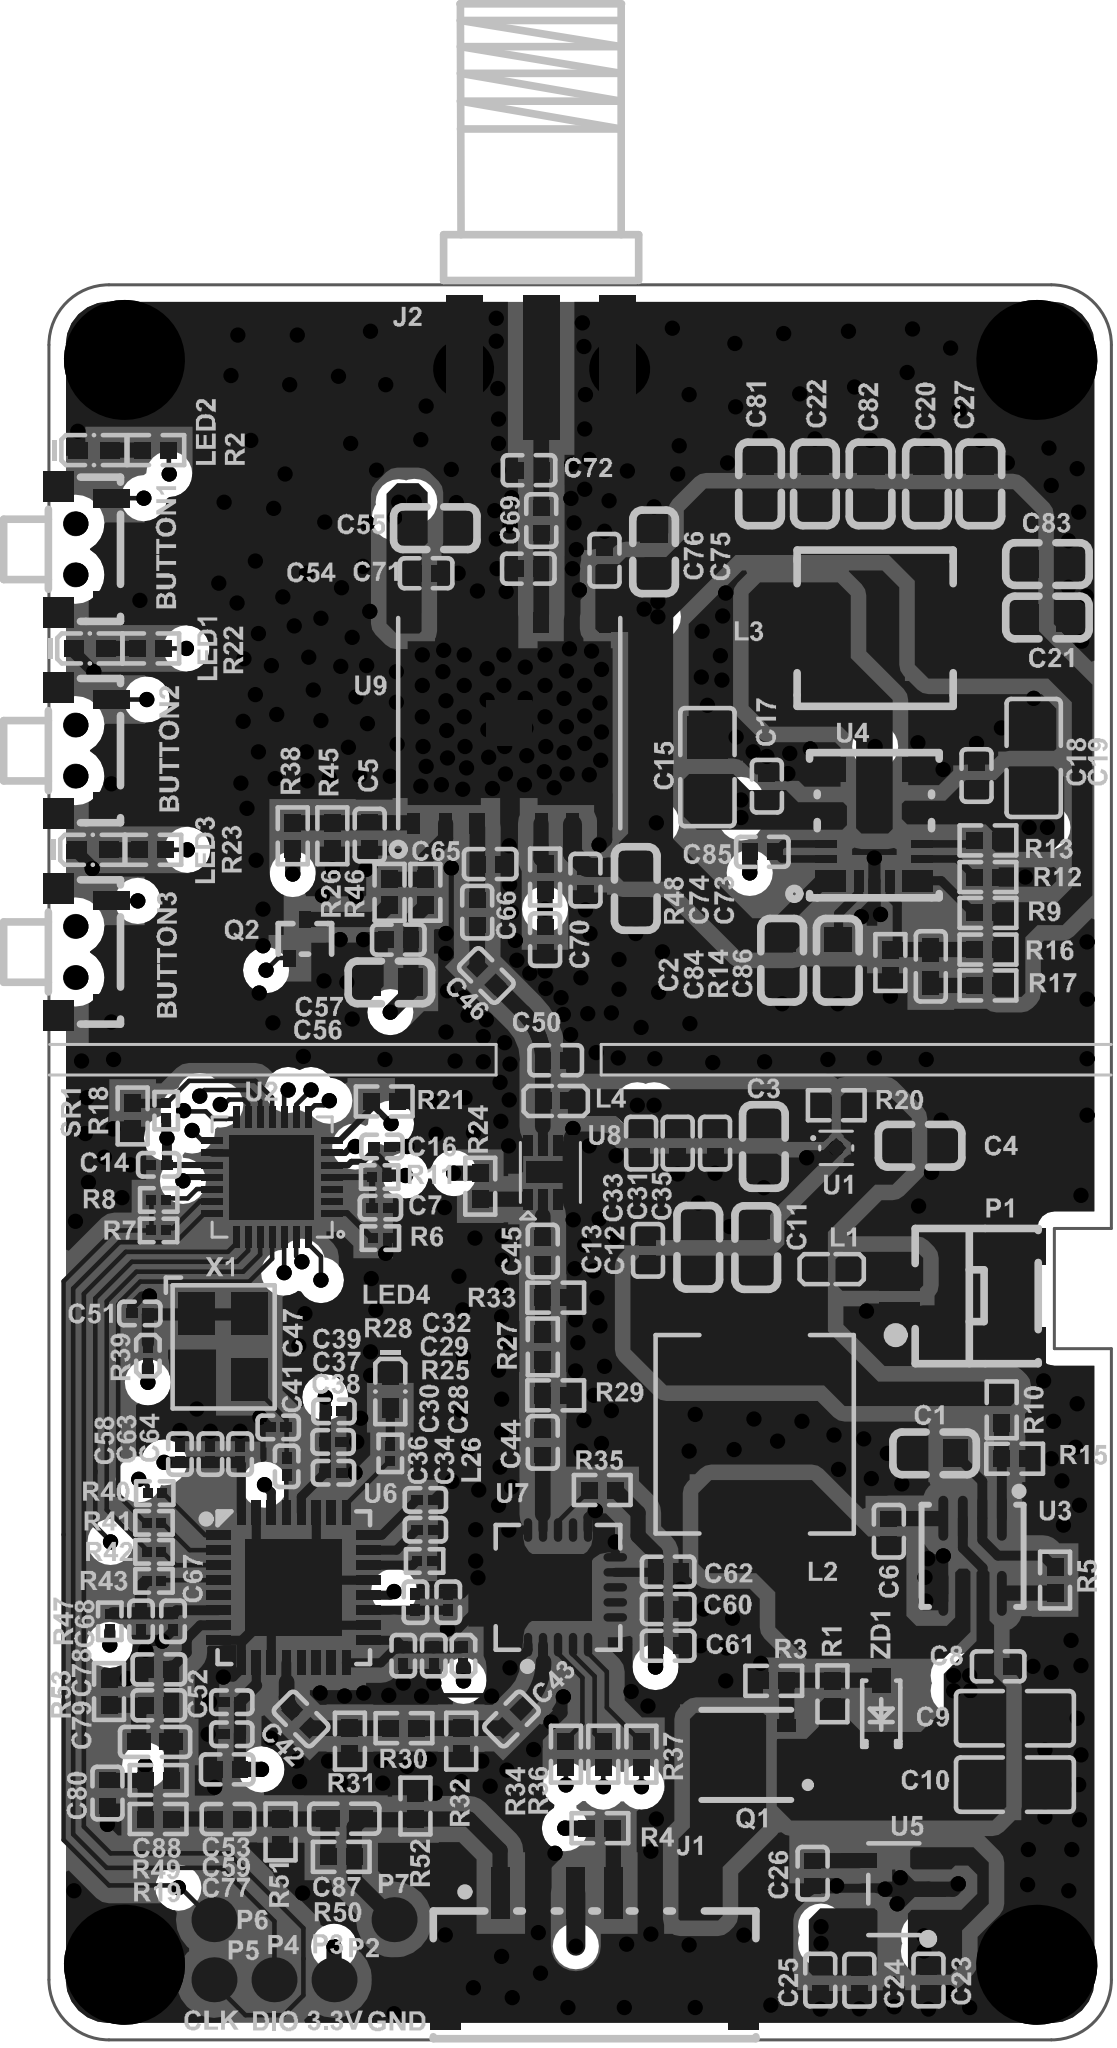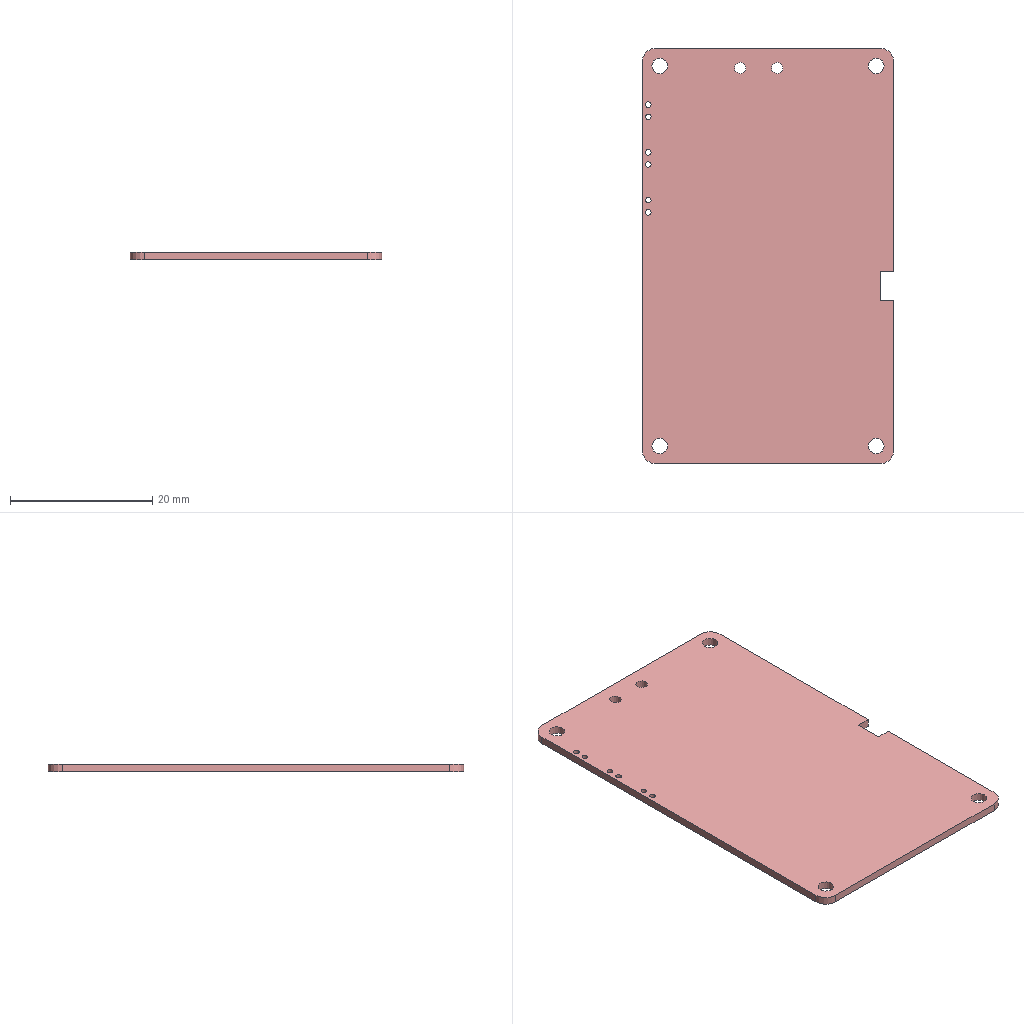Circuit board layout | Altium Designer | box 35.4 x 58.4 x 1.1 mm
Layer stack:
# Altium Designer layer stack of  (unit mm; dielectric type: 0 none, 1 core, 2 prepreg, 3 surface material)
index,name,kind,layer,copper_thickness_mm,dielectric_type,dielectric_thickness_mm,dielectric_material,dielectric_constant
0,Top Paste,other,,,,,,
1,Top Overlay,other,,,,,,
2,Top Solder,dielectric,,,3,0.0102,Solder Resist,3.5
3,Top Layer,copper,Top Layer,0.0356,,,,
4,Dielectric1,dielectric,,,1,0.32,FR-4,4.8
5,Mid-Layer 1,copper,Mid-Layer 1,0.0356,,,,
6,Dielectric2,dielectric,,,2,0.32,FR-4,4.8
7,Mid-Layer 2,copper,Mid-Layer 2,0.0356,,,,
8,Dielectric3,dielectric,,,1,0.32,FR-4,4.8
9,Bottom Layer,copper,Bottom Layer,0.0356,,,,
10,Bottom Solder,dielectric,,,3,0.0102,Solder Resist,3.5
11,Bottom Overlay,other,,,,,,
12,Bottom Paste,other,,,,,,
# drill layer pairs: low layer,high layer
drill_pair,Top Layer,Bottom Layer
Part placement:
Designator,Comment,Layer,Footprint,Center-X(mm),Center-Y(mm),Rotation
R21,10K,TopLayer,R0402,90.5,75.489,360
U9,32A,TopLayer,AU64XX,94.666,88.077,90
P7,Pad,TopLayer,PAD,90.829,48.263,0
P6,Pad,TopLayer,PAD,84.829,48.263,0
R20,NC,TopLayer,R0402,105.562,75.362,360
R19,2K,TopLayer,R0402,82.967,51.613,360
C88,22UF,TopLayer,C0402,82.865,54.178,360
C87,150PF,TopLayer,C0402,89.17,51.623,180
R17,1K,TopLayer,R0402,110.617,79.35,180
C86,22pF,TopLayer,C0402,108.712,79.985,270
U3,AWK6943,TopLayer,QFN-8_L3.0-W3.0-P0.65-BL,110.104,60.37,180
L2,SL0624-100M,TopLayer,IND-SMD_L7.1-W6.6,102.845,64.414,90
C10,10uF,TopLayer,C0805,111.515,52.756,360
C9,10uF,TopLayer,C0805,111.515,54.966,360
R5,100K,TopLayer,R0402,112.852,59.563,270
R15,24.9K,TopLayer,R0402,111.506,63.602,360
R10,107K,TopLayer,R0402,111.074,65.227,270
L1,MPZ1005S121CT000,TopLayer,L0402,105.41,69.901,180
C1,1uf,TopLayer,C0603,108.839,63.779,180
C13,100nf,TopLayer,C0402,99.289,70.536,90
C12,22uF,TopLayer,C0603,100.965,70.637,90
C11,22uF,TopLayer,C0603,102.895,70.626,90
C8,100nf,TopLayer,C0402,110.957,56.693,360
C6,0.1uF,TopLayer,C0402,107.315,61.189,270
C3,1uF,TopLayer,C0603,103.149,73.99,270
C4,1uF,TopLayer,C0603,108.356,74.016,360
C5,0.1uF,TopLayer,C0402,90.018,84.353,90
C7,100nf,TopLayer,C0201,90.373,71.958,180
C14,100nf,TopLayer,C0201,82.987,73.381,180
C16,100nf,TopLayer,C0201,90.424,73.99,360
C23,1uF,TopLayer,C0402,108.636,46.253,270
C24,1uF,TopLayer,C0402,106.333,46.246,270
C25,100nf,TopLayer,C0402,105.029,46.253,270
C26,3.3nf,TopLayer,C0402,104.775,49.809,270
C28,0.1uF,TopLayer,C0201,92.634,58.826,270
C29,0.1uF,TopLayer,C0201,91.872,61.239,360
C30,1NF,TopLayer,C0201,91.542,58.826,90
C31,1UF,TopLayer,C0402,100.279,74.103,90
C32,1NF,TopLayer,C0201,91.872,62.23,180
C33,100nf,TopLayer,C0402,99.06,74.103,90
C34,0.1uF,TopLayer,C0201,92.151,57.048,90
C35,10PF   50V,TopLayer,C0402,101.524,74.103,270
C36,1NF,TopLayer,C0201,91.135,57.048,270
C37,0.1uF,TopLayer,C0201,88.798,64.16,180
C38,1NF,TopLayer,C0201,88.81,63.135,360
C39,0.1uF,TopLayer,C0201,88.824,65.176,180
C41,1NF,TopLayer,C0201,87.249,63.348,90
C42,10PF,TopLayer,C0402,87.732,54.94,315
C43,10PF,TopLayer,C0402,94.742,54.94,45
C44,10PF,TopLayer,C0402,95.783,64.147,90
C45,10PF,TopLayer,C0402,95.783,70.51,90
C46,10PF,TopLayer,C0402,93.904,79.68,135
C47,1NF,TopLayer,C0201,86.97,64.643,180
C50,NC,TopLayer,C0402,96.215,76.86,360
C51,1NF,TopLayer,C0201,82.356,68.436,360
C52,100PF,TopLayer,C0201,85.42,55.499,180
C53,0.1uF,TopLayer,C0201,85.42,54.432,360
C58,1NF,TopLayer,C0201,83.693,63.754,270
C59,10uF,TopLayer,C0402,85.268,53.264,360
C60,1NF,TopLayer,C0402,99.961,58.598,180
C61,100nf,TopLayer,C0402,99.961,57.379,180
C62,1UF,TopLayer,C0402,99.961,59.842,180
C63,1NF,TopLayer,C0201,84.709,63.754,270
C64,1NF,TopLayer,C0201,85.7,63.754,90
C67,1NF,TopLayer,C0201,83.464,58.191,270
C68,0.1uF,TopLayer,C0201,82.398,58.191,90
C77,4.7UF,TopLayer,C0402,85.293,51.613,180
C78,4.7UF,TopLayer,C0402,82.993,56.591,180
C79,22UF,TopLayer,C0402,82.993,55.397,360
C80,2PF,TopLayer,C0402,81.28,52.476,90
R1,50K,TopLayer,R0402,105.435,55.778,270
R2,3.3K,TopLayer,R0402,82.891,97.163,180
R3,100K,TopLayer,R0402,103.48,56.21,360
R4,1K,TopLayer,R0402,97.688,51.308,180
R6,10K,TopLayer,R0201,90.373,70.942,180
R7,22R,TopLayer,R0201,82.982,71.196,180
R8,22R,TopLayer,R0201,82.987,72.212,180
R11,10K,TopLayer,R0201,90.348,72.974,360
R18,10K,TopLayer,R0201,83.236,75.184,90
R22,3.3K,TopLayer,R0402,82.723,90.563,180
R23,3.3K,TopLayer,R0402,82.793,83.863,180
R24,3.9K,TopLayer,R0402,93.701,72.669,270
R25,4.7K,TopLayer,R0201,91.846,60.198,180
R27,30R,TopLayer,R0402,95.783,67.322,90
R28,4.7K,TopLayer,R0201,90.703,63.779,270
R29,180R,TopLayer,R0402,96.215,65.71,360
R30,18R,TopLayer,R0402,91.159,54.635,0
R31,300R,TopLayer,R0402,89.357,54.204,270
R32,300R,TopLayer,R0402,93.066,54.204,270
R33,180R,TopLayer,R0402,96.215,68.961,360
R34,0R,TopLayer,R0402,96.555,53.769,270
R35,0R,TopLayer,R0402,97.765,62.56,360
R36,0R,TopLayer,R0402,97.799,53.769,270
R37,0R,TopLayer,R0402,99.069,53.769,270
R40,0R,TopLayer,R0201,82.855,62.459,180
R41,0R,TopLayer,R0201,82.829,61.468,180
R42,0R,TopLayer,R0201,82.829,60.503,180
R43,0R,TopLayer,R0201,82.829,59.538,180
R47,0R,TopLayer,R0201,81.356,58.191,270
R49,20K,TopLayer,R0402,82.967,52.908,180
R50,270R,TopLayer,R0402,89.068,50.353,360
R51,10R,TopLayer,R0402,87.046,51.181,270
R52,91R,TopLayer,R0402,91.542,52.045,90
R53,22R,TopLayer,R0402,81.331,55.855,90
SR1,SDNT1005X103F3380FTF,TopLayer,R0402,82.118,75.006,270
J1,WAFER-GH1. 25-6PWB,TopLayer,SMD_6P-P1.25_XUNPU_WAFER-GH1.25-6PWB,97.51,47.574,360
BUTTON1,TS24CA250GF013,TopLayer,SW-SMD_L4.7-W3.5-P3.35-EH,80.529,93.863,360
BUTTON2,TS24CA250GF013,TopLayer,SW-SMD_L4.7-W3.5-P3.35-EH,80.529,87.163,360
BUTTON3,TS24CA250GF013,TopLayer,SW-SMD_L4.7-W3.5-P3.35-EH,80.529,80.463,360
U5,RT9013-33GB,TopLayer,SOT-23-5_L3.0-W1.7-P0.95-LS2.8-BL,107.48,49.276,90
U1,TPS7A2050PDQNR,TopLayer,X2SON-4_L1.0-W1.0-P0.65-TL-EP,105.562,73.939,0
U2,GD32E230G8U6,TopLayer,QFN-28_L4.0-W4.0-P0.40-BL-EP2.8,86.766,72.974,90
LED1,LED,TopLayer,LED0402,80.691,90.563,360
LED2,LED,TopLayer,LED0402,80.829,97.163,360
LED3,LED,TopLayer,LED0402,80.791,83.863,360
LED4,LED,TopLayer,LED0402,90.703,65.837,270
SCREW2,MARK_4,TopLayer,M2,81.829,100.163,90
SCREW3,MARK_4,TopLayer,M2,112.229,46.763,90
SCREW4,MARK_4,TopLayer,M2,112.229,100.163,90
P2,Pad,TopLayer,PAD,90.829,46.263,0
P3,Pad,TopLayer,PAD,88.829,46.263,0
P4,Pad,TopLayer,PAD,86.829,46.263,0
P5,Pad,TopLayer,PAD,84.829,46.263,0
X1,OT322525MJBA4SL,TopLayer,SMD3225,85.129,67.343,270
U7,ARW621A,TopLayer,QFN-20_L4.0-W4.0-P0.50-TL-EP2.2,96.291,59.321,90
L4,33nH,TopLayer,L0402,96.215,75.514,360
L26,BLM03PX800SN1D,TopLayer,L0201,93.142,57.048,90
R39,BLM03PX800SN1D,TopLayer,L0201,82.626,67.031,90
P1,WAFER-SHB1.0-2PWB,TopLayer,SMD_2P-WAFER-SHB1.0-2PWB,109.541,69.013,90
ZD1,BZT52C15S,TopLayer,SOD-323_L1.7-W1.3-LS2.6-RD,107.061,55.093,90
Q1,CJAE10P06,TopLayer,DFN-8_L3.0-W3.0-P0.65-BL_G48N03D3,102.54,53.746,90
U6,GX1288FL,TopLayer,QFN-32_L5.0-W5.0-P0.50,87.488,59.309,360
U8,CBG9092,TopLayer,CBG9092,96.037,73.127,90
C17,100nf,TopLayer,C0402,103.251,85.979,90
C18,100nf,TopLayer,C0402,110.236,86.335,90
C85,0.1uF,TopLayer,C0402,103.099,83.795,180
L3,MCS0530-4R7MN2,TopLayer,IND-SMD_L5.2-W5.2_YSPI0530,106.858,91.237,360
R9,100K,TopLayer,R0402,110.617,81.763,360
R12,33.2K,TopLayer,R0402,110.617,82.956,360
R13,10K,TopLayer,R0402,110.617,84.176,360
R14,24.9K,TopLayer,R0402,107.366,80.112,270
R16,113K,TopLayer,R0402,110.617,80.543,180
U4,LM61460AASQRJRRQ1,TopLayer,VQFN-14-HR_L4.0-W3.5-TL_LM61460AASQRJRRQ1,106.832,84.684,90
C2,1uf,TopLayer,C0603,103.759,80.188,270
C20,22uF,TopLayer,C0603,108.585,96.037,90
C21,22uF,TopLayer,C0603,112.598,91.592,360
C22,22uF,TopLayer,C0603,104.851,96.037,90
C27,22uF,TopLayer,C0603,110.363,96.037,90
C81,22uF,TopLayer,C0603,103.022,96.037,90
C82,22uF,TopLayer,C0603,106.705,96.037,90
C83,1uf,TopLayer,C0603,112.598,93.37,360
C84,1uf,TopLayer,C0603,105.613,80.188,270
C15,10uF,TopLayer,C0805,101.27,86.614,90
C19,10uF,TopLayer,C0805,112.141,86.919,90
C54,10PF,TopLayer,C0402,91.897,93.066,360
C55,4.7UF,TopLayer,C0603,92.202,94.564,360
C56,4.7UF,TopLayer,C0603,90.69,79.451,360
C57,10PF,TopLayer,C0402,90.969,80.874,360
C65,NC,TopLayer,C0402,94.031,83.388,360
C66,10PF,TopLayer,C0402,93.599,81.788,270
C69,10PF,TopLayer,C0402,95.733,94.818,90
C70,2.2NF,TopLayer,C0402,95.86,80.874,90
C71,NC,TopLayer,C0402,95.301,93.218,360
C72,NC,TopLayer,C0402,95.326,96.495,360
C73,4.7uF,TopLayer,C0603,98.882,82.575,270
C74,10PF,TopLayer,C0402,97.206,82.855,270
C75,4.7UF,TopLayer,C0603,99.492,93.777,90
C76,10PF,TopLayer,C0402,97.841,93.497,90
R38,0R,TopLayer,R0402,87.452,84.328,90
R45,1MR,TopLayer,R0402,88.773,84.328,270
R46,1K,TopLayer,R0402,91.872,82.448,90
R48,,TopLayer,R0402,95.86,82.956,90
SCREW1,MARK_4,TopLayer,M2,81.829,46.763,90
J2,SMA-50KE-3,TopLayer,SMA-FP-945G,95.729,99.888,90
Q2,DULCTU3134K,TopLayer,SOT-523-3_L1.6-W0.8-P0.50-LS1.6-BR-1,87.859,80.899,270
R26,1K,TopLayer,R0402,90.678,82.448,270
Pad and via stacks:
# Altium Designer via and pad stacks of  (unit mm). Each distinct definition once, with the count of objects using it.
# via: kind,start_layer,end_layer,hole_mm,diameter_mm,mode(0 simple;1 top-mid-bottom;2 full stack),diameter_per_layer,count,example_net
# pad: kind,layer,hole_mm,hole_type(0 round;1 square;2 slot),plating,top_size,top_shape(1 round;2 rect;3 octagon;9 rounded rect),mid_size,bottom_size,mode,footprint,size_per_layer,count,example
pad,Top Layer,0,0,plated,0.5657x0.54,2,0.5657x0.54,0.5657x0.54,0,R0402,,80,R21.2
pad,Top Layer,0,0,plated,1.524x1.524,2,1.524x1.524,1.524x1.524,0,AU64XX,,1,U9.15
pad,Top Layer,0,0,plated,0.675x0.4,2,0.675x0.4,0.675x0.4,0,AU64XX,,12,U9.14
pad,Top Layer,0,0,plated,0.675x0.4999,2,0.675x0.4999,0.675x0.4999,0,AU64XX,,2,U9.10
pad,Top Layer,0,0,plated,4.8x1.2,2,4.8x1.2,4.8x1.2,0,SMA-FP-945G,,3,J2.1
pad,Top Layer,0,0,plated,0.25x0.7,2,0.25x0.7,0.25x0.7,0,VQFN-14-HR_L4.0-W3.5-TL_LM61460AASQRJRRQ1,,4,U4.7
pad,Top Layer,0,0,plated,0.4x1,2,0.4x1,0.4x1,0,VQFN-14-HR_L4.0-W3.5-TL_LM61460AASQRJRRQ1,,2,U4.8
pad,Top Layer,0,0,plated,0.8x1,2,0.8x1,0.8x1,0,VQFN-14-HR_L4.0-W3.5-TL_LM61460AASQRJRRQ1,,2,U4.9
pad,Top Layer,0,0,plated,0.7x1,2,0.7x1,0.7x1,0,VQFN-14-HR_L4.0-W3.5-TL_LM61460AASQRJRRQ1,,2,U4.5
pad,Top Layer,0,0,plated,0.4x2.4,2,0.4x2.4,0.4x2.4,0,VQFN-14-HR_L4.0-W3.5-TL_LM61460AASQRJRRQ1,,1,U4.10
pad,Top Layer,0,0,plated,0.3x0.7,2,0.3x0.7,0.3x0.7,0,VQFN-14-HR_L4.0-W3.5-TL_LM61460AASQRJRRQ1,,3,U4.4
pad,Top Layer,0,0,plated,1.8x2.5,2,1.8x2.5,1.8x2.5,0,IND-SMD_L5.2-W5.2_YSPI0530,,2,L3.2
pad,Top Layer,0,0,plated,0.3x0.67,2,0.3x0.67,0.3x0.67,0,CBG9092,,8,U8.1
pad,Top Layer,0,0,plated,0.7x1.6,2,0.7x1.6,0.7x1.6,0,CBG9092,,1,U8.9
pad,Top Layer,0,0,plated,3.2x3.2,2,3.2x3.2,3.2x3.2,0,QFN-32_L5.0-W5.0-P0.50,,1,U6.33
pad,Top Layer,0,0,plated,0.3x0.8,2,0.3x0.8,0.3x0.8,0,QFN-32_L5.0-W5.0-P0.50,,32,U6.32
pad,Top Layer,0,0,plated,2.6x2,2,2.6x2,2.6x2,0,DFN-8_L3.0-W3.0-P0.65-BL_G48N03D3,,1,Q1.9
pad,Top Layer,0,0,plated,0.4x0.6,2,0.4x0.6,0.4x0.6,0,DFN-8_L3.0-W3.0-P0.65-BL_G48N03D3,,8,Q1.5
pad,Top Layer,0,0,plated,0.63x0.83,2,0.63x0.83,0.63x0.83,0,SOD-323_L1.7-W1.3-LS2.6-RD,,2,ZD1.1
pad,Top Layer,0,0,plated,1.2x2.22,2,1.2x2.22,1.2x2.22,0,SMD_2P-WAFER-SHB1.0-2PWB,,2,P1.4
pad,Top Layer,0,0,plated,0.6x1.35,2,0.6x1.35,0.6x1.35,0,SMD_2P-WAFER-SHB1.0-2PWB,,2,P1.2
pad,Top Layer,0,0,plated,0.3684x0.324,2,0.3684x0.324,0.3684x0.324,0,L0201,,4,L26.1
pad,Top Layer,0,0,plated,2.2x2.2,2,2.2x2.2,2.2x2.2,0,QFN-20_L4.0-W4.0-P0.50-TL-EP2.2,,1,U7.21
pad,Top Layer,0,0,plated,0.28x0.79,1,0.28x0.79,0.28x0.79,0,QFN-20_L4.0-W4.0-P0.50-TL-EP2.2,,10,U7.20
pad,Top Layer,0,0,plated,0.79x0.28,1,0.79x0.28,0.79x0.28,0,QFN-20_L4.0-W4.0-P0.50-TL-EP2.2,,10,U7.15
pad,Top Layer,0,0,plated,1.4x1.2,2,1.4x1.2,1.4x1.2,0,SMD3225,,4,X1.4
pad,Top Layer,0,0,plated,0.6365x0.54,2,0.6365x0.54,0.6365x0.54,0,LED0402,,8,LED1.1
pad,Top Layer,0,0,plated,0.2x0.7,2,0.2x0.7,0.2x0.7,0,QFN-28_L4.0-W4.0-P0.40-BL-EP2.8,,14,U2.4
pad,Top Layer,0,0,plated,0.7x0.2,2,0.7x0.2,0.7x0.2,0,QFN-28_L4.0-W4.0-P0.40-BL-EP2.8,,14,U2.8
pad,Top Layer,0,0,plated,2.8x2.8,2,2.8x2.8,2.8x2.8,0,QFN-28_L4.0-W4.0-P0.40-BL-EP2.8,,1,U2.29
pad,Top Layer,0,0,plated,0.4801x0.4801,2,0.4801x0.4801,0.4801x0.4801,0,X2SON-4_L1.0-W1.0-P0.65-TL-EP,,1,U1.5
pad,Top Layer,0,0,plated,0.1247x0.1247,1,0.1247x0.1247,0.1247x0.1247,0,X2SON-4_L1.0-W1.0-P0.65-TL-EP,,4,U1.4
pad,Top Layer,0,0,plated,0.49x1.157,2,0.49x1.157,0.49x1.157,0,SOT-23-5_L3.0-W1.7-P0.95-LS2.8-BL,,3,U5.1
pad,Top Layer,0,0,plated,0.49x1.175,2,0.49x1.175,0.49x1.175,0,SOT-23-5_L3.0-W1.7-P0.95-LS2.8-BL,,2,U5.4
pad,Top Layer,0,0,plated,0.6x1.2,2,0.6x1.2,0.6x1.2,0,SW-SMD_L4.7-W3.5-P3.35-EH,,6,BUTTON1.2
pad,Top Layer,0,0,plated,1x1,2,1x1,1x1,0,SW-SMD_L4.7-W3.5-P3.35-EH,,6,BUTTON1.3
pad,Top Layer,0,0,plated,1x2.8,2,1x2.8,1x2.8,0,SMD_6P-P1.25_XUNPU_WAFER-GH1.25-6PWB,,2,J1.8
pad,Top Layer,0,0,plated,0.6x1.7,2,0.6x1.7,0.6x1.7,0,SMD_6P-P1.25_XUNPU_WAFER-GH1.25-6PWB,,6,J1.4
pad,Top Layer,0,0,plated,0.3031x0.324,2,0.3031x0.324,0.3031x0.324,0,R0201,,24,R6.2
pad,Top Layer,0,0,plated,0.3684x0.324,2,0.3684x0.324,0.3684x0.324,0,C0201,,44,C7.2
pad,Top Layer,0,0,plated,0.8x0.9,2,0.8x0.9,0.8x0.9,0,C0603,,36,C1.1
pad,Top Layer,0,0,plated,0.54x0.54,2,0.54x0.54,0.54x0.54,0,L0402,,4,L1.2
pad,Top Layer,0,0,plated,1.41x1.35,2,1.41x1.35,1.41x1.35,0,C0805,,8,C10.1
pad,Top Layer,0,0,plated,2.15x3.32,2,2.15x3.32,2.15x3.32,0,IND-SMD_L7.1-W6.6,,2,L2.1
pad,Top Layer,0,0,plated,0.33x1.5,1,0.33x1.5,0.33x1.5,0,QFN-8_L3.0-W3.0-P0.65-BL,,8,U3.1
pad,Top Layer,0,0,plated,0.7901x0.54,2,0.7901x0.54,0.7901x0.54,0,C0402,,6,C88.1
pad,Top Layer,0,0,plated,1.5x1.5,1,1.5x1.5,1.5x1.5,0,PAD,,6,P7.1
pad,Top Layer,0,0,plated,0.5x0.54,2,0.5x0.54,0.5x0.54,0,C0402,,76,C6.1
pad,Top Layer,0,0,plated,0.5334x0.4,2,0.5334x0.4,0.5334x0.4,0,SOT-523-3_L1.6-W0.8-P0.50-LS1.6-BR-1,,1,Q2.3
pad,Top Layer,0,0,plated,0.5334x0.4064,2,0.5334x0.4064,0.5334x0.4064,0,SOT-523-3_L1.6-W0.8-P0.50-LS1.6-BR-1,,2,Q2.2
pad,Multi-Layer,1.6,0,plated,2x2,1,2x2,2x2,0,SMA-FP-945G,,2,J2.2
pad,Multi-Layer,2.2,0,plated,4x4,1,4x4,4x4,0,M2,,4,SCREW2.1
pad,Multi-Layer,0.8,0,unplated,0.8x0.8,1,0.8x0.8,0.8x0.8,0,SW-SMD_L4.7-W3.5-P3.35-EH,,6,BUTTON1.0
pad,Bottom Layer,0,0,plated,4.8x1.2,2,4.8x1.2,4.8x1.2,0,SMA-FP-945G,,2,J2.2
via,Top Layer,Bottom Layer,0.3048,0.508,0,,570,GND
Copper pours:
name,layer,net,type(0 solid;1 hatched;2 none)
Bottom Layer-No Net,Top Layer,PA_5.5V,0
Bottom Layer-No Net,Top Layer,PA_5.5V,0
Bottom Layer-No Net,Top Layer,GND,0
Bottom Layer-No Net,Top Layer,PA_5.5V,0
Bottom Layer-No Net,Top Layer,NetC85_2,0
Bottom Layer-No Net,Top Layer,POWER-IN,0
Bottom Layer-No Net,Top Layer,POWER-IN,0
Bottom Layer-No Net,Top Layer,3.3V,0
Bottom Layer-No Net,Top Layer,VCC_5V,0
Bottom Layer-No Net,Top Layer,VCC_5V3,0
Bottom Layer-No Net,Top Layer,VCC_5V,0
Bottom Layer-No Net,Top Layer,+5V-FAN,0
Bottom Layer-No Net,Top Layer,NetC6_2,0
Bottom Layer-No Net,Top Layer,POWER-IN,0
Bottom Layer-No Net,Top Layer,NetJ1_6,0
Bottom Layer-No Net,Mid-Layer 2,PA_5.5V,0
Bottom Layer-No Net,Mid-Layer 2,GND,0
Bottom Layer-No Net,Mid-Layer 2,POWER-IN,0
Bottom Layer-No Net,Mid-Layer 2,VCC_5V,0
Bottom Layer-No Net,Mid-Layer 2,VCC_5V,0
Bottom Layer-No Net,Mid-Layer 2,3.3V,0
Bottom Layer-No Net,Bottom Layer,GND,0
Bottom Layer-No Net,Mid-Layer 1,GND,0
Design rules, without the lines most boards share:
# Altium Designer design rules of  (exported by Altium Designer, unit mm)
# columns: name | kind | enabled | priority | scope1 | scope2 | descriptor | typed fields (field=value)
Clearance_5 | 0 | enabled | 1 | INPOLYGON | All | Clearance Constraint (Gap=6mil) (INPOLYGON),(All) | gap=0.1524
Clearance | 0 | enabled | 2 | All | All | Clearance Constraint (Gap=6mil) (All),(All) | gap=0.1524
PlaneConnect | 6 | enabled | 1 | All | All | Power Plane Connect Rule(Direct Connect )(Expansion=20mil) (Conductor Width=10mil) (Air Gap=10mil) (Entries=4) (All) | relief_conductor_width=0.254 relief_entries=4 relief_expansion=0.508
PlaneClearance | 12 | enabled | 1 | All | All | Power Plane Clearance (Clearance =6mil) (All) | clearance=0.1524
PolygonConnect | 20 | enabled | 1 | All | All | Polygon Connect Rule(Direct Connect )(Conductor Width=10mil) (Relief Angle=90 Angle) (Entries=4) (Air Gap Width=10mil) (All),(All) | connect_style(0=relief,1=direct,2=none)=1 relief_conductor_width=0.254 relief_entries=4
Width | 2 | enabled | 1 | All | All | Width Constraint (Min=6mil) (Max=100mil) (Preferred=6mil) (All) |
RoutingVias | 11 | enabled | 1 | All | All | Routing Via (MinHoleWidth=12mil) (MaxHoleWidth=12mil) (PreferredHoleWidth=12mil) (MinWidth=20mil) (MaxWidth=20mil) (PreferedWidth=20mil) (All) | via_min_hole=0.3048 via_max_hole=0.3048 via_preferred_diameter=0.508 via_preferred_hole=0.3048
SolderMaskExpansion | 13 | enabled | 1 | All | All | Solder Mask Expansion (Expansion =4mil) (All) | expansion=0.1016
HoleSize | 42 | enabled | 1 | All | All | Hole Size Constraint (Min=1mil) (Max=500mil) (All) |
DiffPairsRouting | 51 | enabled | 1 | All | All | Differential Pairs Uncoupled Length using the Gap Constraints (Min=6mil) (Max=6mil) (Prefered=6mil)  and Width Constraints (Min=15mil) (Max=15mil) (Prefered=15mil) (All) |
HoleToHoleClearance | 52 | enabled | 1 | All | All | Hole To Hole Clearance (Gap=0mil) (All),(All) | gap=0
MinimumSolderMaskSliver | 53 | enabled | 1 | All | All | Minimum Solder Mask Sliver (Gap=0mil) (All),(All) |
SilkscreenOverComponentPads | 54 | enabled | 1 | IsPad | All | Silk To Solder Mask (Clearance=0mil) (IsPad),(All) |
SilkToSilkClearance | 55 | enabled | 1 | All | All | Silk to Silk (Clearance=0mil) (All),(All) |
Classes set for this board:
# Altium Designer classes of  (member kind: 0 net, 1 component, 2 from-to, 3 pad, 4 layer, 5 differential pair, 6 design channel, 7 polygon, 8 structure, 9 xSignal)
# columns: class name | member kind | superclass | members
3.3G_GX1288FL_5W | 1 | no | BUTTON1; BUTTON2; BUTTON3; C3; C4; C5; C6; C7; C8; C9; C10; C11; C12; C13; C14; C15; C16; C17; C18; C19; C20; C21; C22; C23; C24; C25; C26; C27; C28; C29; C30; C31; C32; C33; C34; C35; C36; C37; C38; C39; C41; C42; C43; C44; C45; C46; C47; C50; C51; C52; C53; C54; C55; C56; C57; C58; C59; C60; C61; C62; C63; C64; C65; C66; C67; C68; C69; C70; C71; C72; C73; C74; C75; C76; C77; C78; C79; C80; J1; J2; L1; L2; L3; L4; LED1; LED2; LED3; LED4; P1; P2; P3; P4; P5; Q1; R1; R3; R4; R5; R6; R7; R8; R9; R10; R11; R12; R13; R14; R15; R16; R17; R18; R19; R22; R25; R26; R28; R30; R31; R32; R35; R39; R40; R41; R42; R43; R45; R46; R47; R48; R49; R50; R51; R52; R5; R?; R?; R?; R?; R?; R?; R?; R?; R?; R?; SCREW1; SCREW2; SCREW3; SCREW4; SR1; U1; U2; U3; U4; U5; U6; U7; U8; U9; X1; ZD1; R1; R3; R4; R6; R7; R8; R11; R18; R22; R25; R28; R30; R31; R32; R35; R40; R41; R42; R43; R47; R49; R50; R51; R52; R?; R?; R?; R?; R?; R?; R?; R?; R?; R?; R?; SR1; C3; C4; C5; C7; C14; C16; C23; C24; C25; C26; C28; C29; C30; C31; C32; C33; C34; C35; C36; C37; C38; C39; C41; C42; C43; C44; C45; C46; C47; C50; C51; C52; C53; C58; C59; C60; C61; C62; C63; C64; C67; C68; C77; C78; C79; C80; R1; R2; R3; R4; R6; R7; R8; R11; R18; R22; R23; R24; R25; R27; R28; R29; R30; R31; R32; R33; R34; R35; R36; R37; R40; R41; R42; R43; R47; R49; R50; R51; R52; R53; SR1; J1; BUTTON1; BUTTON2; BUTTON3; U5; U1; U2; LED1; LED2; LED3; LED4; SCREW2; SCREW3; SCREW4; P2; P3; P4; P5; X1; U7; L4; L26; R39; P1; ZD1; Q1; U6; U8; C6; C8; C11; C12; C13; C1; L1; R10; R15; R?; C9; C10; L2; U3; C17; C18; C85; L3; R9; R12; R13; R14; R16; U4; C2; C20; C21; C22; C27; C81; C82; C83; C84; C15; C19; C54; C55; C56; C57; C65; C66; C69; C70; C71; C72; C73; C74; C75; C76; R38; R45; R46; R48; SCREW1; J2; U9; C86; R17; C87; C88; R19; R20; P6; P7; U9; R21; Q2; R26;